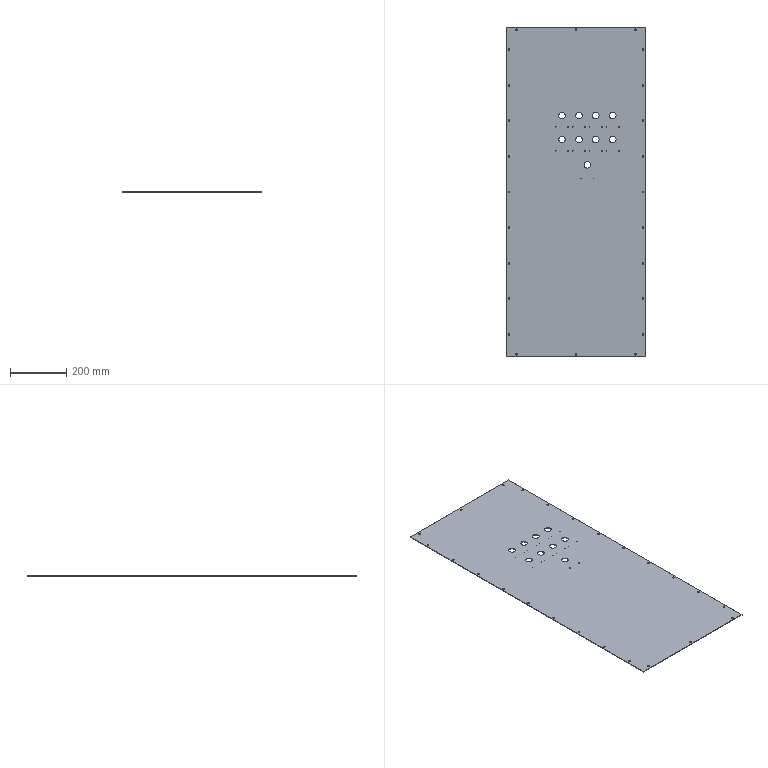Part | SolidWorks | 1 solid | 108 faces | box 494.5 x 1168 x 2 mm | volume 1145967 mm3 | cylinder 102 | plane 6 | commonest cylinder face diameters 6.5 x48 2.3 x36 23 x16 22.5 x2